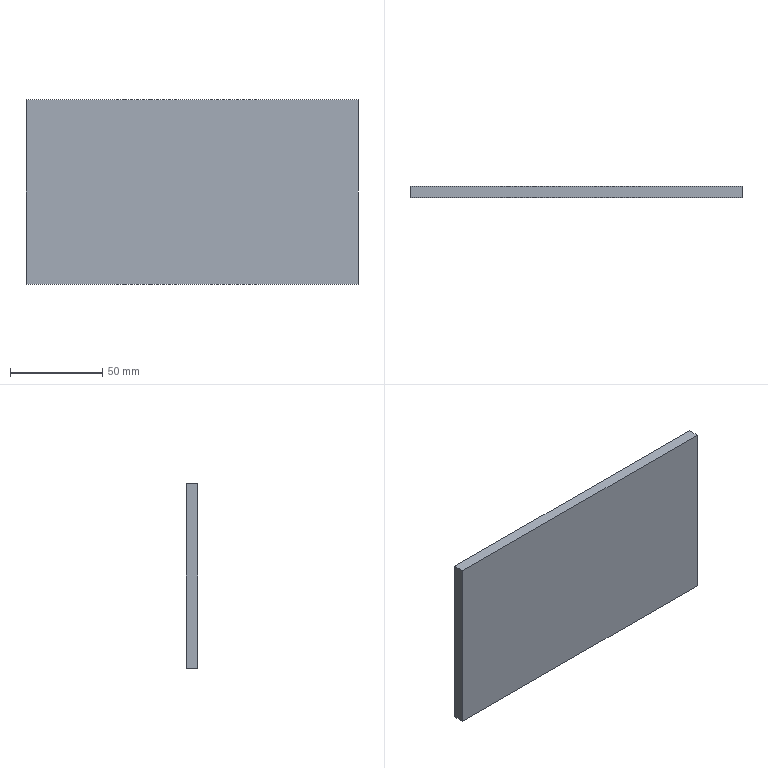Part | SolidWorks | features Extrusion 1 | 1 solid | 6 faces | box 180 x 6 x 100 mm | volume 108000 mm3 | plane 6
STEP:
#1=CARTESIAN_POINT('',(90.,0.,50.));
#2=VERTEX_POINT('',#1);
#3=CARTESIAN_POINT('',(90.,0.,-50.));
#4=VERTEX_POINT('',#3);
#5=CARTESIAN_POINT('',(90.,0.,-50.));
#6=DIRECTION('',(0.,0.,-1.));
#7=VECTOR('',#6,1000.);
#8=LINE('',#5,#7);
#9=EDGE_CURVE('',#2,#4,#8,.T.);
#10=ORIENTED_EDGE('',*,*,#9,.T.);
#11=CARTESIAN_POINT('',(90.,6.,-50.));
#12=VERTEX_POINT('',#11);
#13=CARTESIAN_POINT('',(90.,6.,-50.));
#14=DIRECTION('',(0.,-1.,0.));
#15=VECTOR('',#14,1000.);
#16=LINE('',#13,#15);
#17=EDGE_CURVE('',#12,#4,#16,.T.);
#18=ORIENTED_EDGE('',*,*,#17,.F.);
#19=CARTESIAN_POINT('',(90.,6.,50.));
#20=VERTEX_POINT('',#19);
#21=CARTESIAN_POINT('',(90.,6.,-50.));
#22=DIRECTION('',(0.,0.,-1.));
#23=VECTOR('',#22,1000.);
#24=LINE('',#21,#23);
#25=EDGE_CURVE('',#20,#12,#24,.T.);
#26=ORIENTED_EDGE('',*,*,#25,.F.);
#27=CARTESIAN_POINT('',(90.,6.,50.));
#28=DIRECTION('',(0.,-1.,0.));
#29=VECTOR('',#28,1000.);
#30=LINE('',#27,#29);
#31=EDGE_CURVE('',#20,#2,#30,.T.);
#32=ORIENTED_EDGE('',*,*,#31,.T.);
#33=EDGE_LOOP('',(#10,#18,#26,#32));
#34=FACE_OUTER_BOUND('',#33,.T.);
#35=CARTESIAN_POINT('',(90.,6.,-50.));
#36=DIRECTION('',(-1.,0.,0.));
#37=DIRECTION('',(0.,0.,1.));
#38=AXIS2_PLACEMENT_3D('',#35,#36,#37);
#39=PLANE('',#38);
#40=ADVANCED_FACE('',(#34),#39,.F.);
#41=CARTESIAN_POINT('',(-90.,0.,-50.));
#42=VERTEX_POINT('',#41);
#43=CARTESIAN_POINT('',(-90.,0.,-50.));
#44=DIRECTION('',(-1.,0.,0.));
#45=VECTOR('',#44,1000.);
#46=LINE('',#43,#45);
#47=EDGE_CURVE('',#4,#42,#46,.T.);
#48=ORIENTED_EDGE('',*,*,#47,.T.);
#49=CARTESIAN_POINT('',(-90.,6.,-50.));
#50=VERTEX_POINT('',#49);
#51=CARTESIAN_POINT('',(-90.,6.,-50.));
#52=DIRECTION('',(0.,-1.,0.));
#53=VECTOR('',#52,1000.);
#54=LINE('',#51,#53);
#55=EDGE_CURVE('',#50,#42,#54,.T.);
#56=ORIENTED_EDGE('',*,*,#55,.F.);
#57=CARTESIAN_POINT('',(-90.,6.,-50.));
#58=DIRECTION('',(-1.,0.,0.));
#59=VECTOR('',#58,1000.);
#60=LINE('',#57,#59);
#61=EDGE_CURVE('',#12,#50,#60,.T.);
#62=ORIENTED_EDGE('',*,*,#61,.F.);
#63=ORIENTED_EDGE('',*,*,#17,.T.);
#64=EDGE_LOOP('',(#48,#56,#62,#63));
#65=FACE_OUTER_BOUND('',#64,.T.);
#66=CARTESIAN_POINT('',(-90.,6.,-50.));
#67=DIRECTION('',(0.,0.,1.));
#68=DIRECTION('',(1.,0.,0.));
#69=AXIS2_PLACEMENT_3D('',#66,#67,#68);
#70=PLANE('',#69);
#71=ADVANCED_FACE('',(#65),#70,.F.);
#72=CARTESIAN_POINT('',(-90.,0.,50.));
#73=VERTEX_POINT('',#72);
#74=CARTESIAN_POINT('',(-90.,0.,-50.));
#75=DIRECTION('',(0.,0.,1.));
#76=VECTOR('',#75,1000.);
#77=LINE('',#74,#76);
#78=EDGE_CURVE('',#42,#73,#77,.T.);
#79=ORIENTED_EDGE('',*,*,#78,.T.);
#80=CARTESIAN_POINT('',(-90.,6.,50.));
#81=VERTEX_POINT('',#80);
#82=CARTESIAN_POINT('',(-90.,6.,50.));
#83=DIRECTION('',(0.,-1.,0.));
#84=VECTOR('',#83,1000.);
#85=LINE('',#82,#84);
#86=EDGE_CURVE('',#81,#73,#85,.T.);
#87=ORIENTED_EDGE('',*,*,#86,.F.);
#88=CARTESIAN_POINT('',(-90.,6.,-50.));
#89=DIRECTION('',(0.,0.,1.));
#90=VECTOR('',#89,1000.);
#91=LINE('',#88,#90);
#92=EDGE_CURVE('',#50,#81,#91,.T.);
#93=ORIENTED_EDGE('',*,*,#92,.F.);
#94=ORIENTED_EDGE('',*,*,#55,.T.);
#95=EDGE_LOOP('',(#79,#87,#93,#94));
#96=FACE_OUTER_BOUND('',#95,.T.);
#97=CARTESIAN_POINT('',(-90.,6.,-50.));
#98=DIRECTION('',(1.,0.,0.));
#99=DIRECTION('',(0.,0.,-1.));
#100=AXIS2_PLACEMENT_3D('',#97,#98,#99);
#101=PLANE('',#100);
#102=ADVANCED_FACE('',(#96),#101,.F.);
#103=CARTESIAN_POINT('',(-90.,0.,50.));
#104=DIRECTION('',(1.,0.,0.));
#105=VECTOR('',#104,1000.);
#106=LINE('',#103,#105);
#107=EDGE_CURVE('',#73,#2,#106,.T.);
#108=ORIENTED_EDGE('',*,*,#107,.T.);
#109=ORIENTED_EDGE('',*,*,#31,.F.);
#110=CARTESIAN_POINT('',(-90.,6.,50.));
#111=DIRECTION('',(1.,0.,0.));
#112=VECTOR('',#111,1000.);
#113=LINE('',#110,#112);
#114=EDGE_CURVE('',#81,#20,#113,.T.);
#115=ORIENTED_EDGE('',*,*,#114,.F.);
#116=ORIENTED_EDGE('',*,*,#86,.T.);
#117=EDGE_LOOP('',(#108,#109,#115,#116));
#118=FACE_OUTER_BOUND('',#117,.T.);
#119=CARTESIAN_POINT('',(-90.,6.,50.));
#120=DIRECTION('',(0.,0.,-1.));
#121=DIRECTION('',(-1.,0.,0.));
#122=AXIS2_PLACEMENT_3D('',#119,#120,#121);
#123=PLANE('',#122);
#124=ADVANCED_FACE('',(#118),#123,.F.);
#125=ORIENTED_EDGE('',*,*,#25,.T.);
#126=ORIENTED_EDGE('',*,*,#61,.T.);
#127=ORIENTED_EDGE('',*,*,#92,.T.);
#128=ORIENTED_EDGE('',*,*,#114,.T.);
#129=EDGE_LOOP('',(#125,#126,#127,#128));
#130=FACE_OUTER_BOUND('',#129,.T.);
#131=CARTESIAN_POINT('',(0.,6.,0.));
#132=DIRECTION('',(0.,1.,0.));
#133=DIRECTION('',(0.,0.,1.));
#134=AXIS2_PLACEMENT_3D('',#131,#132,#133);
#135=PLANE('',#134);
#136=ADVANCED_FACE('',(#130),#135,.T.);
#137=ORIENTED_EDGE('',*,*,#9,.F.);
#138=ORIENTED_EDGE('',*,*,#107,.F.);
#139=ORIENTED_EDGE('',*,*,#78,.F.);
#140=ORIENTED_EDGE('',*,*,#47,.F.);
#141=EDGE_LOOP('',(#137,#138,#139,#140));
#142=FACE_OUTER_BOUND('',#141,.T.);
#143=CARTESIAN_POINT('',(0.,0.,0.));
#144=DIRECTION('',(0.,1.,0.));
#145=DIRECTION('',(0.,0.,1.));
#146=AXIS2_PLACEMENT_3D('',#143,#144,#145);
#147=PLANE('',#146);
#148=ADVANCED_FACE('',(#142),#147,.F.);
#149=CLOSED_SHELL('',(#40,#71,#102,#124,#136,#148));
#150=MANIFOLD_SOLID_BREP('',#149);
#151=CARTESIAN_POINT('',(0.,0.,0.));
#152=DIRECTION('',(0.,0.,1.));
#153=DIRECTION('',(1.,0.,0.));
#154=AXIS2_PLACEMENT_3D('',#151,#152,#153);
#155=(LENGTH_UNIT()NAMED_UNIT(*)SI_UNIT(.MILLI.,.METRE.));
#156=UNCERTAINTY_MEASURE_WITH_UNIT(LENGTH_MEASURE(0.00001),#155,'','');
#157=(NAMED_UNIT(*)PLANE_ANGLE_UNIT()SI_UNIT($,.RADIAN.));
#158=(NAMED_UNIT(*)SI_UNIT($,.STERADIAN.)SOLID_ANGLE_UNIT());
#159=(GEOMETRIC_REPRESENTATION_CONTEXT(3)GLOBAL_UNCERTAINTY_ASSIGNED_CONTEXT((#156))GLOBAL_UNIT_ASSIGNED_CONTEXT((#155,#157,#158))REPRESENTATION_CONTEXT('',''));
#160=ADVANCED_BREP_SHAPE_REPRESENTATION('',(#150,#154),#159);